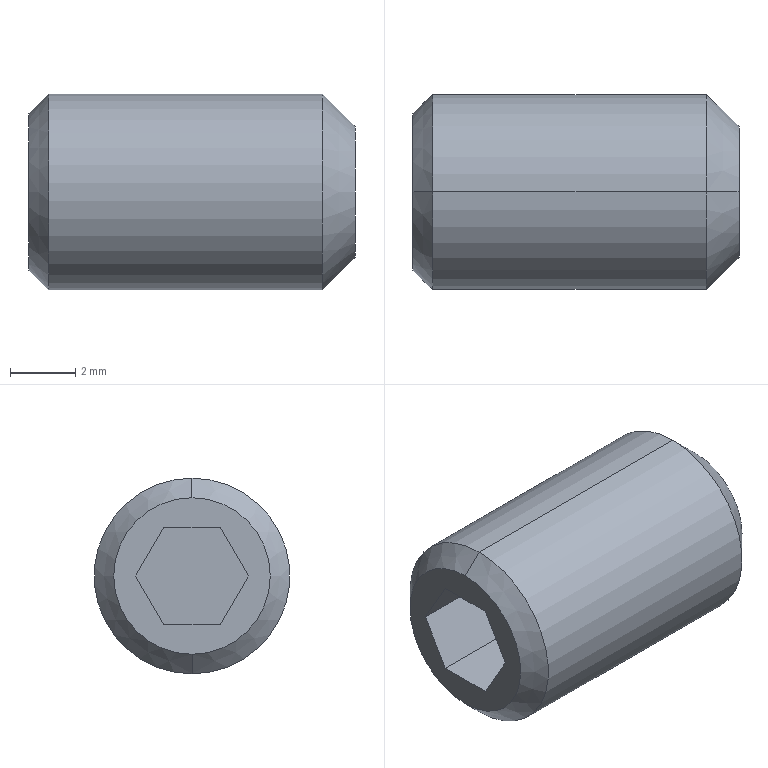Part | STEP file | 00245858_Gewinsestift | 1 solid | 15 faces | box 10 x 6 x 6 mm | volume 243.919 mm3 | plane 9 | cone 4 | cylinder 2 | commonest cylinder face diameters 6 x2
STEP:
#1=CARTESIAN_POINT('',(0.,0.,0.));
#2=DIRECTION('',(0.,0.,1.));
#3=DIRECTION('',(1.,0.,0.));
#4=AXIS2_PLACEMENT_3D('',#1,#2,#3);
#5=CARTESIAN_POINT('',(0.6,0.,-3.));
#6=VERTEX_POINT('',#5);
#7=CARTESIAN_POINT('',(0.6,0.,3.));
#8=VERTEX_POINT('',#7);
#9=CARTESIAN_POINT('',(0.6,0.,0.));
#10=DIRECTION('',(1.,0.,0.));
#11=DIRECTION('',(0.,0.,-1.));
#12=AXIS2_PLACEMENT_3D('',#9,#10,#11);
#13=CIRCLE('',#12,3.);
#14=CARTESIAN_POINT('',(4.8,0.,0.));
#15=DIRECTION('',(1.,0.,0.));
#16=DIRECTION('',(0.,0.,-1.));
#17=AXIS2_PLACEMENT_3D('',#14,#15,#16);
#18=CYLINDRICAL_SURFACE('',#17,3.);
#19=CARTESIAN_POINT('',(0.,-4.2));
#20=DIRECTION('',(1.,0.));
#21=VECTOR('',#20,1.);
#22=LINE('',#19,#21);
#23=(GEOMETRIC_REPRESENTATION_CONTEXT(2)PARAMETRIC_REPRESENTATION_CONTEXT()REPRESENTATION_CONTEXT('',''));
#24=DEFINITIONAL_REPRESENTATION('',(#22),#23);
#25=PCURVE('',#18,#24);
#26=CARTESIAN_POINT('',(0.6,0.,0.));
#27=DIRECTION('',(1.,0.,0.));
#28=DIRECTION('',(0.,0.,-1.));
#29=AXIS2_PLACEMENT_3D('',#26,#27,#28);
#30=CONICAL_SURFACE('',#29,3.,0.7854);
#31=CARTESIAN_POINT('',(0.,0.));
#32=DIRECTION('',(1.,0.));
#33=VECTOR('',#32,1.);
#34=LINE('',#31,#33);
#35=(GEOMETRIC_REPRESENTATION_CONTEXT(2)PARAMETRIC_REPRESENTATION_CONTEXT()REPRESENTATION_CONTEXT('',''));
#36=DEFINITIONAL_REPRESENTATION('',(#34),#35);
#37=PCURVE('',#30,#36);
#38=SURFACE_CURVE('',#13,(#25,#37),.PCURVE_S1.);
#39=EDGE_CURVE('',#6,#8,#38,.T.);
#40=ORIENTED_EDGE('',*,*,#39,.T.);
#41=CARTESIAN_POINT('',(9.,0.,3.));
#42=VERTEX_POINT('',#41);
#43=CARTESIAN_POINT('',(4.8,0.,3.));
#44=DIRECTION('',(1.,0.,0.));
#45=VECTOR('',#44,1.);
#46=LINE('',#43,#45);
#47=CARTESIAN_POINT('',(3.142,0.));
#48=DIRECTION('',(0.,1.));
#49=VECTOR('',#48,1.);
#50=LINE('',#47,#49);
#51=(GEOMETRIC_REPRESENTATION_CONTEXT(2)PARAMETRIC_REPRESENTATION_CONTEXT()REPRESENTATION_CONTEXT('',''));
#52=DEFINITIONAL_REPRESENTATION('',(#50),#51);
#53=PCURVE('',#18,#52);
#54=CARTESIAN_POINT('',(4.8,0.,0.));
#55=DIRECTION('',(1.,0.,0.));
#56=DIRECTION('',(0.,0.,-1.));
#57=AXIS2_PLACEMENT_3D('',#54,#55,#56);
#58=CYLINDRICAL_SURFACE('',#57,3.);
#59=CARTESIAN_POINT('',(3.142,0.));
#60=DIRECTION('',(0.,1.));
#61=VECTOR('',#60,1.);
#62=LINE('',#59,#61);
#63=(GEOMETRIC_REPRESENTATION_CONTEXT(2)PARAMETRIC_REPRESENTATION_CONTEXT()REPRESENTATION_CONTEXT('',''));
#64=DEFINITIONAL_REPRESENTATION('',(#62),#63);
#65=PCURVE('',#58,#64);
#66=SURFACE_CURVE('',#46,(#53,#65),.PCURVE_S1.);
#67=EDGE_CURVE('',#8,#42,#66,.T.);
#68=ORIENTED_EDGE('',*,*,#67,.T.);
#69=CARTESIAN_POINT('',(9.,0.,-3.));
#70=VERTEX_POINT('',#69);
#71=CARTESIAN_POINT('',(9.,0.,0.));
#72=DIRECTION('',(-1.,0.,0.));
#73=DIRECTION('',(0.,0.,-1.));
#74=AXIS2_PLACEMENT_3D('',#71,#72,#73);
#75=CIRCLE('',#74,3.);
#76=CARTESIAN_POINT('',(6.283,4.2));
#77=DIRECTION('',(-1.,0.));
#78=VECTOR('',#77,1.);
#79=LINE('',#76,#78);
#80=(GEOMETRIC_REPRESENTATION_CONTEXT(2)PARAMETRIC_REPRESENTATION_CONTEXT()REPRESENTATION_CONTEXT('',''));
#81=DEFINITIONAL_REPRESENTATION('',(#79),#80);
#82=PCURVE('',#18,#81);
#83=CARTESIAN_POINT('',(9.,0.,0.));
#84=DIRECTION('',(-1.,0.,0.));
#85=DIRECTION('',(0.,0.,1.));
#86=AXIS2_PLACEMENT_3D('',#83,#84,#85);
#87=CONICAL_SURFACE('',#86,3.,0.7854);
#88=CARTESIAN_POINT('',(-3.142,0.));
#89=DIRECTION('',(1.,0.));
#90=VECTOR('',#89,1.);
#91=LINE('',#88,#90);
#92=(GEOMETRIC_REPRESENTATION_CONTEXT(2)PARAMETRIC_REPRESENTATION_CONTEXT()REPRESENTATION_CONTEXT('',''));
#93=DEFINITIONAL_REPRESENTATION('',(#91),#92);
#94=PCURVE('',#87,#93);
#95=SURFACE_CURVE('',#75,(#82,#94),.PCURVE_S1.);
#96=EDGE_CURVE('',#42,#70,#95,.T.);
#97=ORIENTED_EDGE('',*,*,#96,.T.);
#98=CARTESIAN_POINT('',(4.8,0.,-3.));
#99=DIRECTION('',(1.,0.,0.));
#100=VECTOR('',#99,1.);
#101=LINE('',#98,#100);
#102=CARTESIAN_POINT('',(0.,0.));
#103=DIRECTION('',(0.,1.));
#104=VECTOR('',#103,1.);
#105=LINE('',#102,#104);
#106=(GEOMETRIC_REPRESENTATION_CONTEXT(2)PARAMETRIC_REPRESENTATION_CONTEXT()REPRESENTATION_CONTEXT('',''));
#107=DEFINITIONAL_REPRESENTATION('',(#105),#106);
#108=PCURVE('',#18,#107);
#109=CARTESIAN_POINT('',(6.283,0.));
#110=DIRECTION('',(0.,1.));
#111=VECTOR('',#110,1.);
#112=LINE('',#109,#111);
#113=(GEOMETRIC_REPRESENTATION_CONTEXT(2)PARAMETRIC_REPRESENTATION_CONTEXT()REPRESENTATION_CONTEXT('',''));
#114=DEFINITIONAL_REPRESENTATION('',(#112),#113);
#115=PCURVE('',#58,#114);
#116=SURFACE_CURVE('',#101,(#108,#115),.PCURVE_S1.);
#117=EDGE_CURVE('',#6,#70,#116,.T.);
#118=ORIENTED_EDGE('',*,*,#117,.F.);
#119=EDGE_LOOP('',(#40,#68,#97,#118));
#120=FACE_BOUND('',#119,.T.);
#121=ADVANCED_FACE('',(#120),#18,.T.);
#122=CARTESIAN_POINT('',(0.,0.,-2.4));
#123=VERTEX_POINT('',#122);
#124=CARTESIAN_POINT('',(0.,0.,2.4));
#125=VERTEX_POINT('',#124);
#126=CARTESIAN_POINT('',(0.,0.,0.));
#127=DIRECTION('',(1.,0.,0.));
#128=DIRECTION('',(0.,0.,-1.));
#129=AXIS2_PLACEMENT_3D('',#126,#127,#128);
#130=CIRCLE('',#129,2.4);
#131=CARTESIAN_POINT('',(0.,-0.6));
#132=DIRECTION('',(1.,0.));
#133=VECTOR('',#132,1.);
#134=LINE('',#131,#133);
#135=(GEOMETRIC_REPRESENTATION_CONTEXT(2)PARAMETRIC_REPRESENTATION_CONTEXT()REPRESENTATION_CONTEXT('',''));
#136=DEFINITIONAL_REPRESENTATION('',(#134),#135);
#137=PCURVE('',#30,#136);
#138=CARTESIAN_POINT('',(0.,1.2,0.));
#139=DIRECTION('',(1.,0.,0.));
#140=DIRECTION('',(0.,0.,-1.));
#141=AXIS2_PLACEMENT_3D('',#138,#139,#140);
#142=PLANE('',#141);
#143=CARTESIAN_POINT('',(0.,-1.2));
#144=DIRECTION('',(1.,0.));
#145=AXIS2_PLACEMENT_2D('',#143,#144);
#146=CIRCLE('',#145,2.4);
#147=(GEOMETRIC_REPRESENTATION_CONTEXT(2)PARAMETRIC_REPRESENTATION_CONTEXT()REPRESENTATION_CONTEXT('',''));
#148=DEFINITIONAL_REPRESENTATION('',(#146),#147);
#149=PCURVE('',#142,#148);
#150=SURFACE_CURVE('',#130,(#137,#149),.PCURVE_S1.);
#151=EDGE_CURVE('',#123,#125,#150,.T.);
#152=ORIENTED_EDGE('',*,*,#151,.T.);
#153=CARTESIAN_POINT('',(0.6,0.,3.));
#154=DIRECTION('',(0.7071,0.,0.7071));
#155=VECTOR('',#154,1.);
#156=LINE('',#153,#155);
#157=CARTESIAN_POINT('',(3.142,0.));
#158=DIRECTION('',(0.,1.));
#159=VECTOR('',#158,1.);
#160=LINE('',#157,#159);
#161=(GEOMETRIC_REPRESENTATION_CONTEXT(2)PARAMETRIC_REPRESENTATION_CONTEXT()REPRESENTATION_CONTEXT('',''));
#162=DEFINITIONAL_REPRESENTATION('',(#160),#161);
#163=PCURVE('',#30,#162);
#164=CARTESIAN_POINT('',(0.6,0.,0.));
#165=DIRECTION('',(1.,0.,0.));
#166=DIRECTION('',(0.,0.,-1.));
#167=AXIS2_PLACEMENT_3D('',#164,#165,#166);
#168=CONICAL_SURFACE('',#167,3.,0.7854);
#169=CARTESIAN_POINT('',(3.142,0.));
#170=DIRECTION('',(0.,1.));
#171=VECTOR('',#170,1.);
#172=LINE('',#169,#171);
#173=(GEOMETRIC_REPRESENTATION_CONTEXT(2)PARAMETRIC_REPRESENTATION_CONTEXT()REPRESENTATION_CONTEXT('',''));
#174=DEFINITIONAL_REPRESENTATION('',(#172),#173);
#175=PCURVE('',#168,#174);
#176=SURFACE_CURVE('',#156,(#163,#175),.PCURVE_S1.);
#177=EDGE_CURVE('',#125,#8,#176,.T.);
#178=ORIENTED_EDGE('',*,*,#177,.T.);
#179=ORIENTED_EDGE('',*,*,#39,.F.);
#180=CARTESIAN_POINT('',(0.6,0.,-3.));
#181=DIRECTION('',(0.7071,0.,-0.7071));
#182=VECTOR('',#181,1.);
#183=LINE('',#180,#182);
#184=CARTESIAN_POINT('',(0.,0.));
#185=DIRECTION('',(0.,1.));
#186=VECTOR('',#185,1.);
#187=LINE('',#184,#186);
#188=(GEOMETRIC_REPRESENTATION_CONTEXT(2)PARAMETRIC_REPRESENTATION_CONTEXT()REPRESENTATION_CONTEXT('',''));
#189=DEFINITIONAL_REPRESENTATION('',(#187),#188);
#190=PCURVE('',#30,#189);
#191=CARTESIAN_POINT('',(6.283,0.));
#192=DIRECTION('',(0.,1.));
#193=VECTOR('',#192,1.);
#194=LINE('',#191,#193);
#195=(GEOMETRIC_REPRESENTATION_CONTEXT(2)PARAMETRIC_REPRESENTATION_CONTEXT()REPRESENTATION_CONTEXT('',''));
#196=DEFINITIONAL_REPRESENTATION('',(#194),#195);
#197=PCURVE('',#168,#196);
#198=SURFACE_CURVE('',#183,(#190,#197),.PCURVE_S1.);
#199=EDGE_CURVE('',#123,#6,#198,.T.);
#200=ORIENTED_EDGE('',*,*,#199,.F.);
#201=EDGE_LOOP('',(#152,#178,#179,#200));
#202=FACE_BOUND('',#201,.T.);
#203=ADVANCED_FACE('',(#202),#30,.T.);
#204=CARTESIAN_POINT('',(10.,0.,2.));
#205=VERTEX_POINT('',#204);
#206=CARTESIAN_POINT('',(10.,0.,-2.));
#207=VERTEX_POINT('',#206);
#208=CARTESIAN_POINT('',(10.,0.,0.));
#209=DIRECTION('',(-1.,0.,0.));
#210=DIRECTION('',(0.,0.,1.));
#211=AXIS2_PLACEMENT_3D('',#208,#209,#210);
#212=CIRCLE('',#211,2.);
#213=CARTESIAN_POINT('',(0.,-1.));
#214=DIRECTION('',(1.,0.));
#215=VECTOR('',#214,1.);
#216=LINE('',#213,#215);
#217=(GEOMETRIC_REPRESENTATION_CONTEXT(2)PARAMETRIC_REPRESENTATION_CONTEXT()REPRESENTATION_CONTEXT('',''));
#218=DEFINITIONAL_REPRESENTATION('',(#216),#217);
#219=PCURVE('',#87,#218);
#220=CARTESIAN_POINT('',(10.,1.,0.));
#221=DIRECTION('',(1.,0.,0.));
#222=DIRECTION('',(0.,0.,-1.));
#223=AXIS2_PLACEMENT_3D('',#220,#221,#222);
#224=PLANE('',#223);
#225=CARTESIAN_POINT('',(-2.,-1.));
#226=CARTESIAN_POINT('',(-2.,2.464));
#227=CARTESIAN_POINT('',(1.,0.7321));
#228=CARTESIAN_POINT('',(4.,-1.));
#229=CARTESIAN_POINT('',(1.,-2.732));
#230=CARTESIAN_POINT('',(-2.,-4.464));
#231=CARTESIAN_POINT('',(-2.,-1.));
#232=(BOUNDED_CURVE()B_SPLINE_CURVE(2,(#225,#226,#227,#228,#229,#230,#231),.UNSPECIFIED.,.T.,.F.)B_SPLINE_CURVE_WITH_KNOTS((1,2,2,2,2,1),(-2.094,0.,2.094,4.189,6.283,8.378),.UNSPECIFIED.)CURVE()GEOMETRIC_REPRESENTATION_ITEM()RATIONAL_B_SPLINE_CURVE((1.,0.5,1.,0.5,1.,0.5,1.))REPRESENTATION_ITEM(''));
#233=(GEOMETRIC_REPRESENTATION_CONTEXT(2)PARAMETRIC_REPRESENTATION_CONTEXT()REPRESENTATION_CONTEXT('',''));
#234=DEFINITIONAL_REPRESENTATION('',(#232),#233);
#235=PCURVE('',#224,#234);
#236=SURFACE_CURVE('',#212,(#219,#235),.PCURVE_S1.);
#237=EDGE_CURVE('',#205,#207,#236,.T.);
#238=ORIENTED_EDGE('',*,*,#237,.T.);
#239=CARTESIAN_POINT('',(9.,0.,-3.));
#240=DIRECTION('',(-0.7071,0.,-0.7071));
#241=VECTOR('',#240,1.);
#242=LINE('',#239,#241);
#243=CARTESIAN_POINT('',(3.142,0.));
#244=DIRECTION('',(0.,1.));
#245=VECTOR('',#244,1.);
#246=LINE('',#243,#245);
#247=(GEOMETRIC_REPRESENTATION_CONTEXT(2)PARAMETRIC_REPRESENTATION_CONTEXT()REPRESENTATION_CONTEXT('',''));
#248=DEFINITIONAL_REPRESENTATION('',(#246),#247);
#249=PCURVE('',#87,#248);
#250=CARTESIAN_POINT('',(9.,0.,0.));
#251=DIRECTION('',(-1.,0.,0.));
#252=DIRECTION('',(0.,0.,1.));
#253=AXIS2_PLACEMENT_3D('',#250,#251,#252);
#254=CONICAL_SURFACE('',#253,3.,0.7854);
#255=CARTESIAN_POINT('',(3.142,0.));
#256=DIRECTION('',(0.,1.));
#257=VECTOR('',#256,1.);
#258=LINE('',#255,#257);
#259=(GEOMETRIC_REPRESENTATION_CONTEXT(2)PARAMETRIC_REPRESENTATION_CONTEXT()REPRESENTATION_CONTEXT('',''));
#260=DEFINITIONAL_REPRESENTATION('',(#258),#259);
#261=PCURVE('',#254,#260);
#262=SURFACE_CURVE('',#242,(#249,#261),.PCURVE_S1.);
#263=EDGE_CURVE('',#207,#70,#262,.T.);
#264=ORIENTED_EDGE('',*,*,#263,.T.);
#265=ORIENTED_EDGE('',*,*,#96,.F.);
#266=CARTESIAN_POINT('',(9.,0.,3.));
#267=DIRECTION('',(-0.7071,0.,0.7071));
#268=VECTOR('',#267,1.);
#269=LINE('',#266,#268);
#270=CARTESIAN_POINT('',(0.,0.));
#271=DIRECTION('',(0.,1.));
#272=VECTOR('',#271,1.);
#273=LINE('',#270,#272);
#274=(GEOMETRIC_REPRESENTATION_CONTEXT(2)PARAMETRIC_REPRESENTATION_CONTEXT()REPRESENTATION_CONTEXT('',''));
#275=DEFINITIONAL_REPRESENTATION('',(#273),#274);
#276=PCURVE('',#87,#275);
#277=CARTESIAN_POINT('',(6.283,0.));
#278=DIRECTION('',(0.,1.));
#279=VECTOR('',#278,1.);
#280=LINE('',#277,#279);
#281=(GEOMETRIC_REPRESENTATION_CONTEXT(2)PARAMETRIC_REPRESENTATION_CONTEXT()REPRESENTATION_CONTEXT('',''));
#282=DEFINITIONAL_REPRESENTATION('',(#280),#281);
#283=PCURVE('',#254,#282);
#284=SURFACE_CURVE('',#269,(#276,#283),.PCURVE_S1.);
#285=EDGE_CURVE('',#205,#42,#284,.T.);
#286=ORIENTED_EDGE('',*,*,#285,.F.);
#287=EDGE_LOOP('',(#238,#264,#265,#286));
#288=FACE_BOUND('',#287,.T.);
#289=ADVANCED_FACE('',(#288),#87,.T.);
#290=CARTESIAN_POINT('',(3.5,-0.866,-1.5));
#291=VERTEX_POINT('',#290);
#292=CARTESIAN_POINT('',(0.,-0.866,-1.5));
#293=VERTEX_POINT('',#292);
#294=CARTESIAN_POINT('',(0.5,-0.866,-1.5));
#295=DIRECTION('',(-1.,0.,0.));
#296=VECTOR('',#295,1.);
#297=LINE('',#294,#296);
#298=CARTESIAN_POINT('',(0.5,0.,-1.5));
#299=DIRECTION('',(0.,0.,1.));
#300=DIRECTION('',(1.,0.,0.));
#301=AXIS2_PLACEMENT_3D('',#298,#299,#300);
#302=PLANE('',#301);
#303=CARTESIAN_POINT('',(0.,-0.866));
#304=DIRECTION('',(-1.,0.));
#305=VECTOR('',#304,1.);
#306=LINE('',#303,#305);
#307=(GEOMETRIC_REPRESENTATION_CONTEXT(2)PARAMETRIC_REPRESENTATION_CONTEXT()REPRESENTATION_CONTEXT('',''));
#308=DEFINITIONAL_REPRESENTATION('',(#306),#307);
#309=PCURVE('',#302,#308);
#310=CARTESIAN_POINT('',(0.5,-1.299,-0.75));
#311=DIRECTION('',(0.,0.866,0.5));
#312=DIRECTION('',(0.,-0.5,0.866));
#313=AXIS2_PLACEMENT_3D('',#310,#311,#312);
#314=PLANE('',#313);
#315=CARTESIAN_POINT('',(-0.866,0.));
#316=DIRECTION('',(0.,-1.));
#317=VECTOR('',#316,1.);
#318=LINE('',#315,#317);
#319=(GEOMETRIC_REPRESENTATION_CONTEXT(2)PARAMETRIC_REPRESENTATION_CONTEXT()REPRESENTATION_CONTEXT('',''));
#320=DEFINITIONAL_REPRESENTATION('',(#318),#319);
#321=PCURVE('',#314,#320);
#322=SURFACE_CURVE('',#297,(#309,#321),.PCURVE_S1.);
#323=EDGE_CURVE('',#291,#293,#322,.T.);
#324=ORIENTED_EDGE('',*,*,#323,.F.);
#325=CARTESIAN_POINT('',(3.5,0.866,-1.5));
#326=VERTEX_POINT('',#325);
#327=CARTESIAN_POINT('',(3.5,0.,-1.5));
#328=DIRECTION('',(0.,1.,0.));
#329=VECTOR('',#328,1.);
#330=LINE('',#327,#329);
#331=CARTESIAN_POINT('',(3.,0.));
#332=DIRECTION('',(0.,1.));
#333=VECTOR('',#332,1.);
#334=LINE('',#331,#333);
#335=(GEOMETRIC_REPRESENTATION_CONTEXT(2)PARAMETRIC_REPRESENTATION_CONTEXT()REPRESENTATION_CONTEXT('',''));
#336=DEFINITIONAL_REPRESENTATION('',(#334),#335);
#337=PCURVE('',#302,#336);
#338=CARTESIAN_POINT('',(3.5,0.,0.));
#339=DIRECTION('',(1.,0.,0.));
#340=DIRECTION('',(0.,0.,-1.));
#341=AXIS2_PLACEMENT_3D('',#338,#339,#340);
#342=PLANE('',#341);
#343=CARTESIAN_POINT('',(1.5,0.));
#344=DIRECTION('',(0.,1.));
#345=VECTOR('',#344,1.);
#346=LINE('',#343,#345);
#347=(GEOMETRIC_REPRESENTATION_CONTEXT(2)PARAMETRIC_REPRESENTATION_CONTEXT()REPRESENTATION_CONTEXT('',''));
#348=DEFINITIONAL_REPRESENTATION('',(#346),#347);
#349=PCURVE('',#342,#348);
#350=SURFACE_CURVE('',#330,(#337,#349),.PCURVE_S1.);
#351=EDGE_CURVE('',#291,#326,#350,.T.);
#352=ORIENTED_EDGE('',*,*,#351,.T.);
#353=CARTESIAN_POINT('',(0.,0.866,-1.5));
#354=VERTEX_POINT('',#353);
#355=CARTESIAN_POINT('',(0.5,0.866,-1.5));
#356=DIRECTION('',(1.,0.,0.));
#357=VECTOR('',#356,1.);
#358=LINE('',#355,#357);
#359=CARTESIAN_POINT('',(0.,0.866));
#360=DIRECTION('',(1.,0.));
#361=VECTOR('',#360,1.);
#362=LINE('',#359,#361);
#363=(GEOMETRIC_REPRESENTATION_CONTEXT(2)PARAMETRIC_REPRESENTATION_CONTEXT()REPRESENTATION_CONTEXT('',''));
#364=DEFINITIONAL_REPRESENTATION('',(#362),#363);
#365=PCURVE('',#302,#364);
#366=CARTESIAN_POINT('',(0.5,1.299,-0.75));
#367=DIRECTION('',(0.,-0.866,0.5));
#368=DIRECTION('',(0.,-0.5,-0.866));
#369=AXIS2_PLACEMENT_3D('',#366,#367,#368);
#370=PLANE('',#369);
#371=CARTESIAN_POINT('',(0.866,0.));
#372=DIRECTION('',(0.,1.));
#373=VECTOR('',#372,1.);
#374=LINE('',#371,#373);
#375=(GEOMETRIC_REPRESENTATION_CONTEXT(2)PARAMETRIC_REPRESENTATION_CONTEXT()REPRESENTATION_CONTEXT('',''));
#376=DEFINITIONAL_REPRESENTATION('',(#374),#375);
#377=PCURVE('',#370,#376);
#378=SURFACE_CURVE('',#358,(#365,#377),.PCURVE_S1.);
#379=EDGE_CURVE('',#354,#326,#378,.T.);
#380=ORIENTED_EDGE('',*,*,#379,.F.);
#381=CARTESIAN_POINT('',(0.,0.,-1.5));
#382=DIRECTION('',(0.,-1.,0.));
#383=VECTOR('',#382,1.);
#384=LINE('',#381,#383);
#385=CARTESIAN_POINT('',(-0.5,0.));
#386=DIRECTION('',(0.,-1.));
#387=VECTOR('',#386,1.);
#388=LINE('',#385,#387);
#389=(GEOMETRIC_REPRESENTATION_CONTEXT(2)PARAMETRIC_REPRESENTATION_CONTEXT()REPRESENTATION_CONTEXT('',''));
#390=DEFINITIONAL_REPRESENTATION('',(#388),#389);
#391=PCURVE('',#302,#390);
#392=CARTESIAN_POINT('',(1.5,-1.2));
#393=DIRECTION('',(0.,-1.));
#394=VECTOR('',#393,1.);
#395=LINE('',#392,#394);
#396=(GEOMETRIC_REPRESENTATION_CONTEXT(2)PARAMETRIC_REPRESENTATION_CONTEXT()REPRESENTATION_CONTEXT('',''));
#397=DEFINITIONAL_REPRESENTATION('',(#395),#396);
#398=PCURVE('',#142,#397);
#399=SURFACE_CURVE('',#384,(#391,#398),.PCURVE_S1.);
#400=EDGE_CURVE('',#354,#293,#399,.T.);
#401=ORIENTED_EDGE('',*,*,#400,.T.);
#402=EDGE_LOOP('',(#324,#352,#380,#401));
#403=FACE_BOUND('',#402,.T.);
#404=ADVANCED_FACE('',(#403),#302,.T.);
#405=CARTESIAN_POINT('',(3.5,-1.732,0.));
#406=VERTEX_POINT('',#405);
#407=CARTESIAN_POINT('',(0.,-1.732,0.));
#408=VERTEX_POINT('',#407);
#409=CARTESIAN_POINT('',(0.5,-1.732,0.));
#410=DIRECTION('',(-1.,0.,0.));
#411=VECTOR('',#410,1.);
#412=LINE('',#409,#411);
#413=CARTESIAN_POINT('',(0.866,0.));
#414=DIRECTION('',(0.,-1.));
#415=VECTOR('',#414,1.);
#416=LINE('',#413,#415);
#417=(GEOMETRIC_REPRESENTATION_CONTEXT(2)PARAMETRIC_REPRESENTATION_CONTEXT()REPRESENTATION_CONTEXT('',''));
#418=DEFINITIONAL_REPRESENTATION('',(#416),#417);
#419=PCURVE('',#314,#418);
#420=CARTESIAN_POINT('',(0.5,-1.299,0.75));
#421=DIRECTION('',(0.,0.866,-0.5));
#422=DIRECTION('',(0.,0.5,0.866));
#423=AXIS2_PLACEMENT_3D('',#420,#421,#422);
#424=PLANE('',#423);
#425=CARTESIAN_POINT('',(-0.866,0.));
#426=DIRECTION('',(0.,-1.));
#427=VECTOR('',#426,1.);
#428=LINE('',#425,#427);
#429=(GEOMETRIC_REPRESENTATION_CONTEXT(2)PARAMETRIC_REPRESENTATION_CONTEXT()REPRESENTATION_CONTEXT('',''));
#430=DEFINITIONAL_REPRESENTATION('',(#428),#429);
#431=PCURVE('',#424,#430);
#432=SURFACE_CURVE('',#412,(#419,#431),.PCURVE_S1.);
#433=EDGE_CURVE('',#406,#408,#432,.T.);
#434=ORIENTED_EDGE('',*,*,#433,.F.);
#435=CARTESIAN_POINT('',(3.5,-1.299,-0.75));
#436=DIRECTION('',(0.,0.5,-0.866));
#437=VECTOR('',#436,1.);
#438=LINE('',#435,#437);
#439=CARTESIAN_POINT('',(0.,3.));
#440=DIRECTION('',(-1.,0.));
#441=VECTOR('',#440,1.);
#442=LINE('',#439,#441);
#443=(GEOMETRIC_REPRESENTATION_CONTEXT(2)PARAMETRIC_REPRESENTATION_CONTEXT()REPRESENTATION_CONTEXT('',''));
#444=DEFINITIONAL_REPRESENTATION('',(#442),#443);
#445=PCURVE('',#314,#444);
#446=CARTESIAN_POINT('',(0.75,-1.299));
#447=DIRECTION('',(0.866,0.5));
#448=VECTOR('',#447,1.);
#449=LINE('',#446,#448);
#450=(GEOMETRIC_REPRESENTATION_CONTEXT(2)PARAMETRIC_REPRESENTATION_CONTEXT()REPRESENTATION_CONTEXT('',''));
#451=DEFINITIONAL_REPRESENTATION('',(#449),#450);
#452=PCURVE('',#342,#451);
#453=SURFACE_CURVE('',#438,(#445,#452),.PCURVE_S1.);
#454=EDGE_CURVE('',#406,#291,#453,.T.);
#455=ORIENTED_EDGE('',*,*,#454,.T.);
#456=ORIENTED_EDGE('',*,*,#323,.T.);
#457=CARTESIAN_POINT('',(0.,-1.299,-0.75));
#458=DIRECTION('',(0.,-0.5,0.866));
#459=VECTOR('',#458,1.);
#460=LINE('',#457,#459);
#461=CARTESIAN_POINT('',(0.,-0.5));
#462=DIRECTION('',(1.,0.));
#463=VECTOR('',#462,1.);
#464=LINE('',#461,#463);
#465=(GEOMETRIC_REPRESENTATION_CONTEXT(2)PARAMETRIC_REPRESENTATION_CONTEXT()REPRESENTATION_CONTEXT('',''));
#466=DEFINITIONAL_REPRESENTATION('',(#464),#465);
#467=PCURVE('',#314,#466);
#468=CARTESIAN_POINT('',(0.75,-2.499));
#469=DIRECTION('',(-0.866,-0.5));
#470=VECTOR('',#469,1.);
#471=LINE('',#468,#470);
#472=(GEOMETRIC_REPRESENTATION_CONTEXT(2)PARAMETRIC_REPRESENTATION_CONTEXT()REPRESENTATION_CONTEXT('',''));
#473=DEFINITIONAL_REPRESENTATION('',(#471),#472);
#474=PCURVE('',#142,#473);
#475=SURFACE_CURVE('',#460,(#467,#474),.PCURVE_S1.);
#476=EDGE_CURVE('',#293,#408,#475,.T.);
#477=ORIENTED_EDGE('',*,*,#476,.T.);
#478=EDGE_LOOP('',(#434,#455,#456,#477));
#479=FACE_BOUND('',#478,.T.);
#480=ADVANCED_FACE('',(#479),#314,.T.);
#481=ORIENTED_EDGE('',*,*,#379,.T.);
#482=CARTESIAN_POINT('',(3.5,1.732,0.));
#483=VERTEX_POINT('',#482);
#484=CARTESIAN_POINT('',(3.5,1.299,-0.75));
#485=DIRECTION('',(0.,0.5,0.866));
#486=VECTOR('',#485,1.);
#487=LINE('',#484,#486);
#488=CARTESIAN_POINT('',(0.,3.));
#489=DIRECTION('',(-1.,0.));
#490=VECTOR('',#489,1.);
#491=LINE('',#488,#490);
#492=(GEOMETRIC_REPRESENTATION_CONTEXT(2)PARAMETRIC_REPRESENTATION_CONTEXT()REPRESENTATION_CONTEXT('',''));
#493=DEFINITIONAL_REPRESENTATION('',(#491),#492);
#494=PCURVE('',#370,#493);
#495=CARTESIAN_POINT('',(0.75,1.299));
#496=DIRECTION('',(-0.866,0.5));
#497=VECTOR('',#496,1.);
#498=LINE('',#495,#497);
#499=(GEOMETRIC_REPRESENTATION_CONTEXT(2)PARAMETRIC_REPRESENTATION_CONTEXT()REPRESENTATION_CONTEXT('',''));
#500=DEFINITIONAL_REPRESENTATION('',(#498),#499);
#501=PCURVE('',#342,#500);
#502=SURFACE_CURVE('',#487,(#494,#501),.PCURVE_S1.);
#503=EDGE_CURVE('',#326,#483,#502,.T.);
#504=ORIENTED_EDGE('',*,*,#503,.T.);
#505=CARTESIAN_POINT('',(0.,1.732,0.));
#506=VERTEX_POINT('',#505);
#507=CARTESIAN_POINT('',(0.5,1.732,0.));
#508=DIRECTION('',(1.,0.,0.));
#509=VECTOR('',#508,1.);
#510=LINE('',#507,#509);
#511=CARTESIAN_POINT('',(-0.866,0.));
#512=DIRECTION('',(0.,1.));
#513=VECTOR('',#512,1.);
#514=LINE('',#511,#513);
#515=(GEOMETRIC_REPRESENTATION_CONTEXT(2)PARAMETRIC_REPRESENTATION_CONTEXT()REPRESENTATION_CONTEXT('',''));
#516=DEFINITIONAL_REPRESENTATION('',(#514),#515);
#517=PCURVE('',#370,#516);
#518=CARTESIAN_POINT('',(0.5,1.299,0.75));
#519=DIRECTION('',(0.,-0.866,-0.5));
#520=DIRECTION('',(0.,0.5,-0.866));
#521=AXIS2_PLACEMENT_3D('',#518,#519,#520);
#522=PLANE('',#521);
#523=CARTESIAN_POINT('',(0.866,0.));
#524=DIRECTION('',(0.,1.));
#525=VECTOR('',#524,1.);
#526=LINE('',#523,#525);
#527=(GEOMETRIC_REPRESENTATION_CONTEXT(2)PARAMETRIC_REPRESENTATION_CONTEXT()REPRESENTATION_CONTEXT('',''));
#528=DEFINITIONAL_REPRESENTATION('',(#526),#527);
#529=PCURVE('',#522,#528);
#530=SURFACE_CURVE('',#510,(#517,#529),.PCURVE_S1.);
#531=EDGE_CURVE('',#506,#483,#530,.T.);
#532=ORIENTED_EDGE('',*,*,#531,.F.);
#533=CARTESIAN_POINT('',(0.,1.299,-0.75));
#534=DIRECTION('',(0.,-0.5,-0.866));
#535=VECTOR('',#534,1.);
#536=LINE('',#533,#535);
#537=CARTESIAN_POINT('',(0.,-0.5));
#538=DIRECTION('',(1.,0.));
#539=VECTOR('',#538,1.);
#540=LINE('',#537,#539);
#541=(GEOMETRIC_REPRESENTATION_CONTEXT(2)PARAMETRIC_REPRESENTATION_CONTEXT()REPRESENTATION_CONTEXT('',''));
#542=DEFINITIONAL_REPRESENTATION('',(#540),#541);
#543=PCURVE('',#370,#542);
#544=CARTESIAN_POINT('',(0.75,0.09904));
#545=DIRECTION('',(0.866,-0.5));
#546=VECTOR('',#545,1.);
#547=LINE('',#544,#546);
#548=(GEOMETRIC_REPRESENTATION_CONTEXT(2)PARAMETRIC_REPRESENTATION_CONTEXT()REPRESENTATION_CONTEXT('',''));
#549=DEFINITIONAL_REPRESENTATION('',(#547),#548);
#550=PCURVE('',#142,#549);
#551=SURFACE_CURVE('',#536,(#543,#550),.PCURVE_S1.);
#552=EDGE_CURVE('',#506,#354,#551,.T.);
#553=ORIENTED_EDGE('',*,*,#552,.T.);
#554=EDGE_LOOP('',(#481,#504,#532,#553));
#555=FACE_BOUND('',#554,.T.);
#556=ADVANCED_FACE('',(#555),#370,.T.);
#557=CARTESIAN_POINT('',(3.5,-0.866,1.5));
#558=VERTEX_POINT('',#557);
#559=CARTESIAN_POINT('',(0.,-0.866,1.5));
#560=VERTEX_POINT('',#559);
#561=CARTESIAN_POINT('',(0.5,-0.866,1.5));
#562=DIRECTION('',(-1.,0.,0.));
#563=VECTOR('',#562,1.);
#564=LINE('',#561,#563);
#565=CARTESIAN_POINT('',(0.866,0.));
#566=DIRECTION('',(0.,-1.));
#567=VECTOR('',#566,1.);
#568=LINE('',#565,#567);
#569=(GEOMETRIC_REPRESENTATION_CONTEXT(2)PARAMETRIC_REPRESENTATION_CONTEXT()REPRESENTATION_CONTEXT('',''));
#570=DEFINITIONAL_REPRESENTATION('',(#568),#569);
#571=PCURVE('',#424,#570);
#572=CARTESIAN_POINT('',(0.5,0.,1.5));
#573=DIRECTION('',(0.,0.,-1.));
#574=DIRECTION('',(-1.,0.,0.));
#575=AXIS2_PLACEMENT_3D('',#572,#573,#574);
#576=PLANE('',#575);
#577=CARTESIAN_POINT('',(0.,-0.866));
#578=DIRECTION('',(1.,0.));
#579=VECTOR('',#578,1.);
#580=LINE('',#577,#579);
#581=(GEOMETRIC_REPRESENTATION_CONTEXT(2)PARAMETRIC_REPRESENTATION_CONTEXT()REPRESENTATION_CONTEXT('',''));
#582=DEFINITIONAL_REPRESENTATION('',(#580),#581);
#583=PCURVE('',#576,#582);
#584=SURFACE_CURVE('',#564,(#571,#583),.PCURVE_S1.);
#585=EDGE_CURVE('',#558,#560,#584,.T.);
#586=ORIENTED_EDGE('',*,*,#585,.F.);
#587=CARTESIAN_POINT('',(3.5,-0.866,1.5));
#588=DIRECTION('',(0.,-0.5,-0.866));
#589=VECTOR('',#588,1.);
#590=LINE('',#587,#589);
#591=CARTESIAN_POINT('',(0.866,3.));
#592=DIRECTION('',(-1.,0.));
#593=VECTOR('',#592,1.);
#594=LINE('',#591,#593);
#595=(GEOMETRIC_REPRESENTATION_CONTEXT(2)PARAMETRIC_REPRESENTATION_CONTEXT()REPRESENTATION_CONTEXT('',''));
#596=DEFINITIONAL_REPRESENTATION('',(#594),#595);
#597=PCURVE('',#424,#596);
#598=CARTESIAN_POINT('',(-1.5,-0.866));
#599=DIRECTION('',(0.866,-0.5));
#600=VECTOR('',#599,1.);
#601=LINE('',#598,#600);
#602=(GEOMETRIC_REPRESENTATION_CONTEXT(2)PARAMETRIC_REPRESENTATION_CONTEXT()REPRESENTATION_CONTEXT('',''));
#603=DEFINITIONAL_REPRESENTATION('',(#601),#602);
#604=PCURVE('',#342,#603);
#605=SURFACE_CURVE('',#590,(#597,#604),.PCURVE_S1.);
#606=EDGE_CURVE('',#558,#406,#605,.T.);
#607=ORIENTED_EDGE('',*,*,#606,.T.);
#608=ORIENTED_EDGE('',*,*,#433,.T.);
#609=CARTESIAN_POINT('',(0.,-1.299,0.75));
#610=DIRECTION('',(0.,0.5,0.866));
#611=VECTOR('',#610,1.);
#612=LINE('',#609,#611);
#613=CARTESIAN_POINT('',(0.,-0.5));
#614=DIRECTION('',(1.,0.));
#615=VECTOR('',#614,1.);
#616=LINE('',#613,#615);
#617=(GEOMETRIC_REPRESENTATION_CONTEXT(2)PARAMETRIC_REPRESENTATION_CONTEXT()REPRESENTATION_CONTEXT('',''));
#618=DEFINITIONAL_REPRESENTATION('',(#616),#617);
#619=PCURVE('',#424,#618);
#620=CARTESIAN_POINT('',(-0.75,-2.499));
#621=DIRECTION('',(-0.866,0.5));
#622=VECTOR('',#621,1.);
#623=LINE('',#620,#622);
#624=(GEOMETRIC_REPRESENTATION_CONTEXT(2)PARAMETRIC_REPRESENTATION_CONTEXT()REPRESENTATION_CONTEXT('',''));
#625=DEFINITIONAL_REPRESENTATION('',(#623),#624);
#626=PCURVE('',#142,#625);
#627=SURFACE_CURVE('',#612,(#619,#626),.PCURVE_S1.);
#628=EDGE_CURVE('',#408,#560,#627,.T.);
#629=ORIENTED_EDGE('',*,*,#628,.T.);
#630=EDGE_LOOP('',(#586,#607,#608,#629));
#631=FACE_BOUND('',#630,.T.);
#632=ADVANCED_FACE('',(#631),#424,.T.);
#633=ORIENTED_EDGE('',*,*,#531,.T.);
#634=CARTESIAN_POINT('',(3.5,0.866,1.5));
#635=VERTEX_POINT('',#634);
#636=CARTESIAN_POINT('',(3.5,1.732,-0.000000001));
#637=DIRECTION('',(0.,-0.5,0.866));
#638=VECTOR('',#637,1.);
#639=LINE('',#636,#638);
#640=CARTESIAN_POINT('',(0.866,3.));
#641=DIRECTION('',(-1.,0.));
#642=VECTOR('',#641,1.);
#643=LINE('',#640,#642);
#644=(GEOMETRIC_REPRESENTATION_CONTEXT(2)PARAMETRIC_REPRESENTATION_CONTEXT()REPRESENTATION_CONTEXT('',''));
#645=DEFINITIONAL_REPRESENTATION('',(#643),#644);
#646=PCURVE('',#522,#645);
#647=CARTESIAN_POINT('',(0.000000001,1.732));
#648=DIRECTION('',(-0.866,-0.5));
#649=VECTOR('',#648,1.);
#650=LINE('',#647,#649);
#651=(GEOMETRIC_REPRESENTATION_CONTEXT(2)PARAMETRIC_REPRESENTATION_CONTEXT()REPRESENTATION_CONTEXT('',''));
#652=DEFINITIONAL_REPRESENTATION('',(#650),#651);
#653=PCURVE('',#342,#652);
#654=SURFACE_CURVE('',#639,(#646,#653),.PCURVE_S1.);
#655=EDGE_CURVE('',#483,#635,#654,.T.);
#656=ORIENTED_EDGE('',*,*,#655,.T.);
#657=CARTESIAN_POINT('',(0.,0.866,1.5));
#658=VERTEX_POINT('',#657);
#659=CARTESIAN_POINT('',(0.5,0.866,1.5));
#660=DIRECTION('',(1.,0.,0.));
#661=VECTOR('',#660,1.);
#662=LINE('',#659,#661);
#663=CARTESIAN_POINT('',(-0.866,0.));
#664=DIRECTION('',(0.,1.));
#665=VECTOR('',#664,1.);
#666=LINE('',#663,#665);
#667=(GEOMETRIC_REPRESENTATION_CONTEXT(2)PARAMETRIC_REPRESENTATION_CONTEXT()REPRESENTATION_CONTEXT('',''));
#668=DEFINITIONAL_REPRESENTATION('',(#666),#667);
#669=PCURVE('',#522,#668);
#670=CARTESIAN_POINT('',(0.,0.866));
#671=DIRECTION('',(-1.,0.));
#672=VECTOR('',#671,1.);
#673=LINE('',#670,#672);
#674=(GEOMETRIC_REPRESENTATION_CONTEXT(2)PARAMETRIC_REPRESENTATION_CONTEXT()REPRESENTATION_CONTEXT('',''));
#675=DEFINITIONAL_REPRESENTATION('',(#673),#674);
#676=PCURVE('',#576,#675);
#677=SURFACE_CURVE('',#662,(#669,#676),.PCURVE_S1.);
#678=EDGE_CURVE('',#658,#635,#677,.T.);
#679=ORIENTED_EDGE('',*,*,#678,.F.);
#680=CARTESIAN_POINT('',(0.,1.299,0.75));
#681=DIRECTION('',(0.,0.5,-0.866));
#682=VECTOR('',#681,1.);
#683=LINE('',#680,#682);
#684=CARTESIAN_POINT('',(0.,-0.5));
#685=DIRECTION('',(1.,0.));
#686=VECTOR('',#685,1.);
#687=LINE('',#684,#686);
#688=(GEOMETRIC_REPRESENTATION_CONTEXT(2)PARAMETRIC_REPRESENTATION_CONTEXT()REPRESENTATION_CONTEXT('',''));
#689=DEFINITIONAL_REPRESENTATION('',(#687),#688);
#690=PCURVE('',#522,#689);
#691=CARTESIAN_POINT('',(-0.75,0.09904));
#692=DIRECTION('',(0.866,0.5));
#693=VECTOR('',#692,1.);
#694=LINE('',#691,#693);
#695=(GEOMETRIC_REPRESENTATION_CONTEXT(2)PARAMETRIC_REPRESENTATION_CONTEXT()REPRESENTATION_CONTEXT('',''));
#696=DEFINITIONAL_REPRESENTATION('',(#694),#695);
#697=PCURVE('',#142,#696);
#698=SURFACE_CURVE('',#683,(#690,#697),.PCURVE_S1.);
#699=EDGE_CURVE('',#658,#506,#698,.T.);
#700=ORIENTED_EDGE('',*,*,#699,.T.);
#701=EDGE_LOOP('',(#633,#656,#679,#700));
#702=FACE_BOUND('',#701,.T.);
#703=ADVANCED_FACE('',(#702),#522,.T.);
#704=ORIENTED_EDGE('',*,*,#606,.F.);
#705=CARTESIAN_POINT('',(3.5,0.,1.5));
#706=DIRECTION('',(0.,-1.,0.));
#707=VECTOR('',#706,1.);
#708=LINE('',#705,#707);
#709=CARTESIAN_POINT('',(-1.5,0.));
#710=DIRECTION('',(0.,-1.));
#711=VECTOR('',#710,1.);
#712=LINE('',#709,#711);
#713=(GEOMETRIC_REPRESENTATION_CONTEXT(2)PARAMETRIC_REPRESENTATION_CONTEXT()REPRESENTATION_CONTEXT('',''));
#714=DEFINITIONAL_REPRESENTATION('',(#712),#713);
#715=PCURVE('',#342,#714);
#716=CARTESIAN_POINT('',(-3.,0.));
#717=DIRECTION('',(0.,-1.));
#718=VECTOR('',#717,1.);
#719=LINE('',#716,#718);
#720=(GEOMETRIC_REPRESENTATION_CONTEXT(2)PARAMETRIC_REPRESENTATION_CONTEXT()REPRESENTATION_CONTEXT('',''));
#721=DEFINITIONAL_REPRESENTATION('',(#719),#720);
#722=PCURVE('',#576,#721);
#723=SURFACE_CURVE('',#708,(#715,#722),.PCURVE_S1.);
#724=EDGE_CURVE('',#635,#558,#723,.T.);
#725=ORIENTED_EDGE('',*,*,#724,.F.);
#726=ORIENTED_EDGE('',*,*,#655,.F.);
#727=ORIENTED_EDGE('',*,*,#503,.F.);
#728=ORIENTED_EDGE('',*,*,#351,.F.);
#729=ORIENTED_EDGE('',*,*,#454,.F.);
#730=EDGE_LOOP('',(#704,#725,#726,#727,#728,#729));
#731=FACE_BOUND('',#730,.T.);
#732=ADVANCED_FACE('',(#731),#342,.F.);
#733=ORIENTED_EDGE('',*,*,#237,.F.);
#734=CARTESIAN_POINT('',(10.,0.,0.));
#735=DIRECTION('',(-1.,0.,0.));
#736=DIRECTION('',(0.,0.,1.));
#737=AXIS2_PLACEMENT_3D('',#734,#735,#736);
#738=CIRCLE('',#737,2.);
#739=CARTESIAN_POINT('',(-2.,-1.));
#740=CARTESIAN_POINT('',(-2.,2.464));
#741=CARTESIAN_POINT('',(1.,0.7321));
#742=CARTESIAN_POINT('',(4.,-1.));
#743=CARTESIAN_POINT('',(1.,-2.732));
#744=CARTESIAN_POINT('',(-2.,-4.464));
#745=CARTESIAN_POINT('',(-2.,-1.));
#746=(BOUNDED_CURVE()B_SPLINE_CURVE(2,(#739,#740,#741,#742,#743,#744,#745),.UNSPECIFIED.,.T.,.F.)B_SPLINE_CURVE_WITH_KNOTS((1,2,2,2,2,1),(-2.094,0.,2.094,4.189,6.283,8.378),.UNSPECIFIED.)CURVE()GEOMETRIC_REPRESENTATION_ITEM()RATIONAL_B_SPLINE_CURVE((1.,0.5,1.,0.5,1.,0.5,1.))REPRESENTATION_ITEM(''));
#747=(GEOMETRIC_REPRESENTATION_CONTEXT(2)PARAMETRIC_REPRESENTATION_CONTEXT()REPRESENTATION_CONTEXT('',''));
#748=DEFINITIONAL_REPRESENTATION('',(#746),#747);
#749=PCURVE('',#224,#748);
#750=CARTESIAN_POINT('',(0.,-1.));
#751=DIRECTION('',(1.,0.));
#752=VECTOR('',#751,1.);
#753=LINE('',#750,#752);
#754=(GEOMETRIC_REPRESENTATION_CONTEXT(2)PARAMETRIC_REPRESENTATION_CONTEXT()REPRESENTATION_CONTEXT('',''));
#755=DEFINITIONAL_REPRESENTATION('',(#753),#754);
#756=PCURVE('',#254,#755);
#757=SURFACE_CURVE('',#738,(#749,#756),.PCURVE_S1.);
#758=EDGE_CURVE('',#207,#205,#757,.T.);
#759=ORIENTED_EDGE('',*,*,#758,.F.);
#760=EDGE_LOOP('',(#733,#759));
#761=FACE_BOUND('',#760,.T.);
#762=ADVANCED_FACE('',(#761),#224,.T.);
#763=ORIENTED_EDGE('',*,*,#678,.T.);
#764=ORIENTED_EDGE('',*,*,#724,.T.);
#765=ORIENTED_EDGE('',*,*,#585,.T.);
#766=CARTESIAN_POINT('',(0.,1.2,1.5));
#767=DIRECTION('',(0.,1.,0.));
#768=VECTOR('',#767,1.);
#769=LINE('',#766,#768);
#770=CARTESIAN_POINT('',(0.5,1.2));
#771=DIRECTION('',(0.,1.));
#772=VECTOR('',#771,1.);
#773=LINE('',#770,#772);
#774=(GEOMETRIC_REPRESENTATION_CONTEXT(2)PARAMETRIC_REPRESENTATION_CONTEXT()REPRESENTATION_CONTEXT('',''));
#775=DEFINITIONAL_REPRESENTATION('',(#773),#774);
#776=PCURVE('',#576,#775);
#777=CARTESIAN_POINT('',(-1.5,0.));
#778=DIRECTION('',(0.,1.));
#779=VECTOR('',#778,1.);
#780=LINE('',#777,#779);
#781=(GEOMETRIC_REPRESENTATION_CONTEXT(2)PARAMETRIC_REPRESENTATION_CONTEXT()REPRESENTATION_CONTEXT('',''));
#782=DEFINITIONAL_REPRESENTATION('',(#780),#781);
#783=PCURVE('',#142,#782);
#784=SURFACE_CURVE('',#769,(#776,#783),.PCURVE_S1.);
#785=EDGE_CURVE('',#560,#658,#784,.T.);
#786=ORIENTED_EDGE('',*,*,#785,.T.);
#787=EDGE_LOOP('',(#763,#764,#765,#786));
#788=FACE_BOUND('',#787,.T.);
#789=ADVANCED_FACE('',(#788),#576,.T.);
#790=ORIENTED_EDGE('',*,*,#628,.F.);
#791=ORIENTED_EDGE('',*,*,#476,.F.);
#792=ORIENTED_EDGE('',*,*,#400,.F.);
#793=ORIENTED_EDGE('',*,*,#552,.F.);
#794=ORIENTED_EDGE('',*,*,#699,.F.);
#795=ORIENTED_EDGE('',*,*,#785,.F.);
#796=EDGE_LOOP('',(#790,#791,#792,#793,#794,#795));
#797=FACE_BOUND('',#796,.T.);
#798=ORIENTED_EDGE('',*,*,#151,.F.);
#799=CARTESIAN_POINT('',(0.,0.,0.));
#800=DIRECTION('',(1.,0.,0.));
#801=DIRECTION('',(0.,0.,-1.));
#802=AXIS2_PLACEMENT_3D('',#799,#800,#801);
#803=CIRCLE('',#802,2.4);
#804=CARTESIAN_POINT('',(0.,-1.2));
#805=DIRECTION('',(1.,0.));
#806=AXIS2_PLACEMENT_2D('',#804,#805);
#807=CIRCLE('',#806,2.4);
#808=(GEOMETRIC_REPRESENTATION_CONTEXT(2)PARAMETRIC_REPRESENTATION_CONTEXT()REPRESENTATION_CONTEXT('',''));
#809=DEFINITIONAL_REPRESENTATION('',(#807),#808);
#810=PCURVE('',#142,#809);
#811=CARTESIAN_POINT('',(0.,-0.6));
#812=DIRECTION('',(1.,0.));
#813=VECTOR('',#812,1.);
#814=LINE('',#811,#813);
#815=(GEOMETRIC_REPRESENTATION_CONTEXT(2)PARAMETRIC_REPRESENTATION_CONTEXT()REPRESENTATION_CONTEXT('',''));
#816=DEFINITIONAL_REPRESENTATION('',(#814),#815);
#817=PCURVE('',#168,#816);
#818=SURFACE_CURVE('',#803,(#810,#817),.PCURVE_S1.);
#819=EDGE_CURVE('',#125,#123,#818,.T.);
#820=ORIENTED_EDGE('',*,*,#819,.F.);
#821=EDGE_LOOP('',(#798,#820));
#822=FACE_BOUND('',#821,.T.);
#823=ADVANCED_FACE('',(#797,#822),#142,.F.);
#824=ORIENTED_EDGE('',*,*,#263,.F.);
#825=ORIENTED_EDGE('',*,*,#758,.T.);
#826=ORIENTED_EDGE('',*,*,#285,.T.);
#827=CARTESIAN_POINT('',(9.,0.,0.));
#828=DIRECTION('',(-1.,0.,0.));
#829=DIRECTION('',(0.,0.,-1.));
#830=AXIS2_PLACEMENT_3D('',#827,#828,#829);
#831=CIRCLE('',#830,3.);
#832=CARTESIAN_POINT('',(3.142,0.));
#833=DIRECTION('',(1.,0.));
#834=VECTOR('',#833,1.);
#835=LINE('',#832,#834);
#836=(GEOMETRIC_REPRESENTATION_CONTEXT(2)PARAMETRIC_REPRESENTATION_CONTEXT()REPRESENTATION_CONTEXT('',''));
#837=DEFINITIONAL_REPRESENTATION('',(#835),#836);
#838=PCURVE('',#254,#837);
#839=CARTESIAN_POINT('',(6.283,4.2));
#840=DIRECTION('',(-1.,0.));
#841=VECTOR('',#840,1.);
#842=LINE('',#839,#841);
#843=(GEOMETRIC_REPRESENTATION_CONTEXT(2)PARAMETRIC_REPRESENTATION_CONTEXT()REPRESENTATION_CONTEXT('',''));
#844=DEFINITIONAL_REPRESENTATION('',(#842),#843);
#845=PCURVE('',#58,#844);
#846=SURFACE_CURVE('',#831,(#838,#845),.PCURVE_S1.);
#847=EDGE_CURVE('',#70,#42,#846,.T.);
#848=ORIENTED_EDGE('',*,*,#847,.F.);
#849=EDGE_LOOP('',(#824,#825,#826,#848));
#850=FACE_BOUND('',#849,.T.);
#851=ADVANCED_FACE('',(#850),#254,.T.);
#852=ORIENTED_EDGE('',*,*,#177,.F.);
#853=ORIENTED_EDGE('',*,*,#819,.T.);
#854=ORIENTED_EDGE('',*,*,#199,.T.);
#855=CARTESIAN_POINT('',(0.6,0.,0.));
#856=DIRECTION('',(1.,0.,0.));
#857=DIRECTION('',(0.,0.,-1.));
#858=AXIS2_PLACEMENT_3D('',#855,#856,#857);
#859=CIRCLE('',#858,3.);
#860=CARTESIAN_POINT('',(0.,0.));
#861=DIRECTION('',(1.,0.));
#862=VECTOR('',#861,1.);
#863=LINE('',#860,#862);
#864=(GEOMETRIC_REPRESENTATION_CONTEXT(2)PARAMETRIC_REPRESENTATION_CONTEXT()REPRESENTATION_CONTEXT('',''));
#865=DEFINITIONAL_REPRESENTATION('',(#863),#864);
#866=PCURVE('',#168,#865);
#867=CARTESIAN_POINT('',(0.,-4.2));
#868=DIRECTION('',(1.,0.));
#869=VECTOR('',#868,1.);
#870=LINE('',#867,#869);
#871=(GEOMETRIC_REPRESENTATION_CONTEXT(2)PARAMETRIC_REPRESENTATION_CONTEXT()REPRESENTATION_CONTEXT('',''));
#872=DEFINITIONAL_REPRESENTATION('',(#870),#871);
#873=PCURVE('',#58,#872);
#874=SURFACE_CURVE('',#859,(#866,#873),.PCURVE_S1.);
#875=EDGE_CURVE('',#8,#6,#874,.T.);
#876=ORIENTED_EDGE('',*,*,#875,.F.);
#877=EDGE_LOOP('',(#852,#853,#854,#876));
#878=FACE_BOUND('',#877,.T.);
#879=ADVANCED_FACE('',(#878),#168,.T.);
#880=ORIENTED_EDGE('',*,*,#67,.F.);
#881=ORIENTED_EDGE('',*,*,#875,.T.);
#882=ORIENTED_EDGE('',*,*,#117,.T.);
#883=ORIENTED_EDGE('',*,*,#847,.T.);
#884=EDGE_LOOP('',(#880,#881,#882,#883));
#885=FACE_BOUND('',#884,.T.);
#886=ADVANCED_FACE('',(#885),#58,.T.);
#887=CLOSED_SHELL('',(#121,#203,#289,#404,#480,#556,#632,#703,#732,#762,#789,#823,#851,#879,#886));
#888=MANIFOLD_SOLID_BREP('',#887);
#889=(LENGTH_UNIT()NAMED_UNIT(*)SI_UNIT(.MILLI.,.METRE.));
#890=UNCERTAINTY_MEASURE_WITH_UNIT(LENGTH_MEASURE(0.0000001),#889,'','');
#891=(NAMED_UNIT(*)PLANE_ANGLE_UNIT()SI_UNIT($,.RADIAN.));
#892=(NAMED_UNIT(*)SI_UNIT($,.STERADIAN.)SOLID_ANGLE_UNIT());
#893=(GEOMETRIC_REPRESENTATION_CONTEXT(3)GLOBAL_UNCERTAINTY_ASSIGNED_CONTEXT((#890))GLOBAL_UNIT_ASSIGNED_CONTEXT((#889,#891,#892))REPRESENTATION_CONTEXT('',''));
#894=ADVANCED_BREP_SHAPE_REPRESENTATION('',(#4,#888),#893);